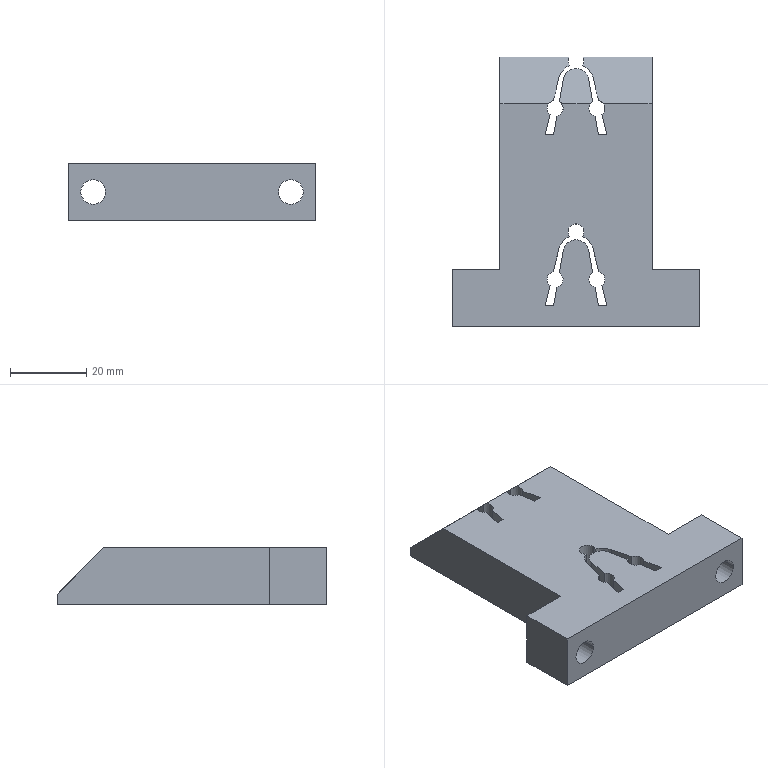Part | STEP file | guide pin seat | 1 solid | 62 faces | box 65 x 71 x 15 mm | volume 41839 mm3 | plane 34 | cylinder 28 | commonest cylinder face diameters 4.2 x18 6.5 x4 9.2 x4 6.8 x2